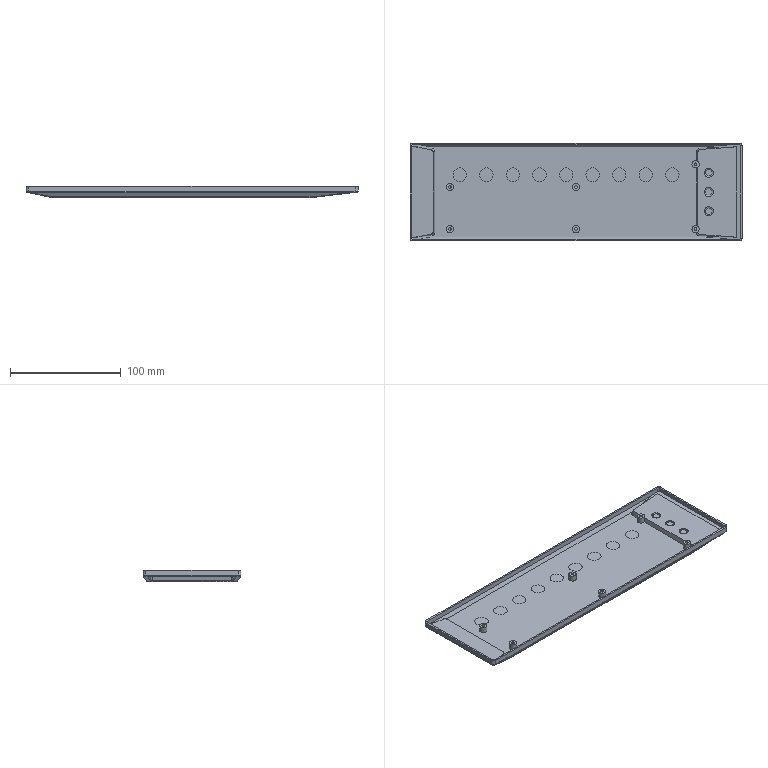NC program | NX | posted with a generic post | part box 300 x 88.5 x 10 mm
Whole program:
N10 G17 G21 G94 G90
(FIXED_CONTOUR_COPY_COPY , TOOL : D3R0.5)
N12 T09 M6
N14 G54
N16 G17 G0 G90 X-99.283 Y37.112 S9500 M3
N18 G43 Z30. H9
N20 Z3.6
N22 G94 G1 Z0.07 F1000.
N24 G3 X-99.023 Y36.962 R0.3
N26 G1 X-98.891 Z0.058 F2500.
N28 X117.392 Y36.963
N30 X117.548 Z0.07
N32 X117.664 Y36.874 Z0.069
N34 X117.542 Z0.057
N36 X117.392 Z0.045
N38 X117.321 Z0.044
N40 X-98.838 Y36.873
N42 X-99.15 Z0.071
N44 X-99.277 Y36.785
N46 X-98.953 Z0.041
N48 X-98.793 Z0.029
N50 X117.233 Y36.786
N52 X117.392 Z0.033
N54 X117.494 Z0.04
N56 X117.779 Z0.069
N58 X117.894 Y36.698 Z0.07
N60 X117.392 Z0.02
N62 X117.144 Z0.015
N64 X-98.749 Y36.697
N66 X-99.046 Z0.037
N68 X-99.404 Z0.072
N70 X-99.53 Y36.61
N72 X-99.041 Z0.025
N74 X-98.705 Z0.
N76 X117.056 Y36.611
N78 X117.409 Z0.009
N80 X118.009 Z0.07
N82 X118.123 Y36.524
N84 X117.35 Z-0.009
N86 X117.08 Z-0.014
N88 X-98.7 Y36.523
N90 X-98.777 Z-0.006
N92 X-99.046 Z0.014
N94 X-99.655 Z0.072
N96 X-99.78 Y36.436
N98 X-99.046 Z0.002
N100 X-98.865 Z-0.012
N102 X-98.7 Z-0.029
N104 X117.12 Y36.437
N106 X117.302 Z-0.025
N108 X118.236 Z0.071
N110 X118.349 Y36.351
N112 X117.255 Z-0.041
N114 X117.159 Z-0.043
N116 X-98.697 Y36.35
N118 X-98.951 Z-0.017
N120 X-99.046 Z-0.01
N122 X-99.904 Z0.072
N124 X-100.027 Y36.264
N126 X-98.67 Z-0.057
N128 X117.208 Y36.265
N130 X118.461 Z0.071
N132 X118.573 Y36.18 Z0.072
N134 X117.177 Z-0.072
N136 X-98.643 Y36.179
N138 X-100.15 Z0.072
N140 X-100.273 Y36.094 Z0.073
N142 X-98.616 Z-0.086
N144 X117.147 Y36.095
N146 X118.684 Z0.072
N148 X118.795 Y36.01
N150 X117.118 Z-0.1
N152 X-98.59 Y36.009
N154 X-100.395 Z0.073
N156 X-100.516 Y35.925
N158 X-98.563 Z-0.114
N160 X117.089 Y35.926
N162 X118.903 Z0.072
N164 X119.012 Y35.842
N166 X117.06 Z-0.128
N168 X-98.536 Y35.841
N170 X-100.636 Z0.073
N172 X-100.756 Y35.757
N174 X-98.51 Z-0.142
N176 X117.031
N178 X119.12 Z0.072
N180 X119.228 Y35.673
N182 X117.002 Z-0.156
N184 X-98.483 Y35.672
N186 X-100.876 Z0.073
N188 X-100.996 Y35.588
N190 X-98.456 Z-0.17
N192 X116.973 Y35.589
N194 X119.337 Z0.072
N196 X119.446 Y35.504 Z0.073
N198 X116.944 Z-0.184
N200 X-98.43
N202 X-101.116 Z0.073
N204 X-101.236 Y35.419
N206 X-98.403 Z-0.198
N208 X116.915 Y35.42
N210 X119.554 Z0.073
N212 X119.663 Y35.336
N214 X116.886 Z-0.212
N216 X-98.376 Y35.335
N218 X-101.356 Z0.073
N220 X-101.477 Y35.25
N222 X-98.35 Z-0.226
N224 X116.857 Y35.251
N226 X119.771 Z0.073
N228 X119.88 Y35.166
N230 X116.828 Z-0.24
N232 X-98.323 Z-0.241
N234 X-101.597 Z0.073
N236 X-101.717 Y35.081
N238 X-98.296 Z-0.255
N240 X116.799 Y35.082 Z-0.254
N242 X119.988 Z0.073
N244 X120.096 Y34.997
N246 X116.769 Z-0.269
N248 X-98.269 Y34.996
N250 X-101.838 Z0.073
N252 X-101.959 Y34.911
N254 X-98.243 Z-0.283
N256 X116.74 Y34.912
N258 X120.205 Z0.073
N260 X120.314 Y34.827
N262 X116.711 Z-0.297
N264 X-98.216
N266 X-102.079 Z0.073
N268 X-102.2 Y34.742
N270 X-98.189 Z-0.311
N272 X116.682 Y34.743
N274 X120.422 Z0.073
N276 X120.531 Y34.658
N278 X116.653 Z-0.325
N280 X-98.162 Y34.657
N282 X-102.321 Z0.073
N284 X-102.441 Y34.571
N286 X-98.135 Z-0.34
N288 X116.623 Y34.572 Z-0.339
N290 X120.64 Z0.073
N292 X120.749 Y34.486
N294 X116.594 Z-0.354
N296 X-98.107 Y34.485
N298 X-102.562 Z0.073
N300 X-102.684 Y34.399 Z0.072
N302 X-98.081 Z-0.368
N304 X116.564 Y34.4
N306 X120.858 Z0.072
N308 X120.969 Y34.313
N310 X116.534 Z-0.383
N312 X-98.053 Y34.312
N314 X-102.807 Z0.072
N316 X-102.93 Y34.224
N318 X-98.026 Z-0.397
N320 X116.504 Y34.225
N322 X121.079 Z0.072
N324 X121.191 Y34.138
N326 X116.474 Y34.137 Z-0.412
N328 X-97.998
N330 X-103.054 Z0.072
N332 X-103.178 Y34.048
N334 X-97.97 Z-0.427
N336 X116.443 Y34.049
N338 X121.302 Z0.072
N340 X121.414 Y33.961
N342 X116.413 Z-0.441
N344 X-97.942 Y33.96
N346 X-103.303 Z0.072
N348 X-103.427 Y33.871
N350 X-97.913 Z-0.456
N352 X116.382 Y33.872
N354 X121.527 Z0.072
N356 X121.638 Y33.784
N358 X116.352 Z-0.471
N360 X-97.886 Y33.783
N362 X-103.552 Z0.072
N364 X-103.676 Y33.695 Z0.071
N366 X-97.858 Z-0.486
N368 X116.321 Y33.696 Z-0.485
N370 X121.75 Z0.071
N372 X121.862 Y33.608
N374 X116.291 Z-0.5
N376 X-97.831 Y33.607
N378 X-103.799 Z0.071
N380 X-103.922 Y33.519
N382 X-97.803 Z-0.515
N384 X116.261 Y33.52
N386 X121.972 Z0.071
N388 X122.082 Y33.432
N390 X116.231 Z-0.529
N392 X-97.77 Y33.431
N394 X-104.044 Z0.071
N396 X-104.166 Y33.344 Z0.07
N398 X-97.894 Z-0.53
N400 X-97.735 Z-0.544
N402 X116.201 Y33.345
N404 X122.192 Z0.071
N406 X122.301 Y33.258 Z0.07
N408 X116.171 Z-0.558
N410 X-97.701 Y33.257
N412 X-97.947 Z-0.537
N414 X-104.288 Z0.07
N416 X-104.409 Y33.17
N418 X-97.999 Z-0.543
N420 X-97.666 Z-0.572
N422 X116.142 Y33.171
N424 X122.41 Z0.07
N426 X122.518 Y33.085
N428 X116.109 Z-0.586
N430 X-97.661 Y33.084 Z-0.587
N432 X-104.529 Z0.07
N434 X-104.65 Y32.998 Z0.069
N436 X-97.732 Z-0.592
N438 G3 X-97.472 Y33.148 R0.3
N440 G1 Z2.558
N442 G0 Z3.158
N444 X-98.024 Y32.941
N446 Z2.558
N448 G1 Z-0.592 F1000.
N450 G3 X-97.784 Y32.961 R0.24
N452 G1 X-97.773 Y32.97 F2500.
N454 X-97.855 Y32.912
N456 X-104.769 Z0.069
N458 X-104.888 Y32.827
N460 X-97.977 Z-0.592
N462 X-98.098 Y32.742
N464 X-105.007 Z0.069
N466 X-105.124 Y32.656 Z0.068
N468 X-98.221 Z-0.592
N470 X-98.345 Y32.57
N472 X-105.241 Z0.068
N474 X-105.284 Y32.537
N476 X-105.335 Y32.495 Z0.066
N478 X-105.353 Y32.479 Z0.067
N480 X-98.474 Z-0.592
N482 X-98.614 Y32.382
N484 X-105.177 Y32.381 Z0.037
N486 X-105.366 Z0.068
N488 X-105.369 Y32.282
N490 X-104.984 Z0.004
N492 X-98.755 Z-0.592
N494 X-98.897 Y32.183
N496 X-104.793 Z-0.027
N498 X-105.371 Z0.068
N500 X-105.372 Y32.084
N502 X-104.603 Z-0.059
N504 X-99.038 Z-0.592
N506 X-99.179 Y31.985
N508 X-104.413 Z-0.09
N510 X-105.373 Z0.068
N512 X-105.374 Y31.886 Z0.069
N514 X-104.222 Z-0.121
N516 X-102.751 Z-0.264
N518 X-99.319 Z-0.592
N520 X-99.46 Y31.787
N522 X-103.914 Z-0.166
N524 X-104.031 Z-0.153
N526 X-104.933 Z-0.004
N528 X-105.375 Z0.069
N530 X-105.376 Y31.688
N532 X-103.86 Z-0.181
N534 X-103.764 Z-0.193
N536 X-99.601 Z-0.592
N538 X-99.742 Y31.589
N540 X-103.442 Z-0.237
N542 X-103.651 Z-0.216
N544 X-105.377 Z0.069
N546 X-105.378 Y31.49
N548 X-103.46 Z-0.248
N550 X-103.256 Z-0.269
N552 X-99.883 Z-0.592
N554 X-100.024 Y31.391
N556 X-103.141 Z-0.294
N558 X-103.269 Z-0.28
N560 X-104.195 Z-0.127
N562 X-105.379 Z0.07
N564 X-105.38 Y31.292
N566 X-103.077 Z-0.312
N568 X-100.165 Z-0.592
N570 X-100.305 Y31.193
N572 X-102.887 Z-0.344
N574 X-105.381 Z0.07
N576 X-105.382 Y31.093
N578 X-102.698 Z-0.377
N580 X-100.445 Z-0.592
N582 X-100.585 Y30.994
N584 X-102.505 Z-0.409
N586 X-105.383 Z0.07
N588 X-105.384 Y30.895
N590 X-102.315 Z-0.441
N592 X-100.725 Z-0.592
N594 X-100.865 Y30.796
N596 X-102.124 Z-0.472
N598 X-105.385 Z0.071
N600 X-105.386 Y30.697
N602 X-101.934 Z-0.504
N604 X-101.006 Z-0.592
N606 X-101.145 Y30.598
N608 X-101.744 Z-0.535
N610 X-105.387 Z0.071
N612 Y30.499
N614 X-101.554 Z-0.567
N616 X-101.285 Z-0.593
N618 X-101.402 Y30.416 Z-0.592
N620 Y30.4
N622 X-105.388 Y30.399 Z0.071
N624 X-105.389 Y30.299
N626 X-101.402 Y30.3 Z-0.592
N628 X-101.403 Y30.2
N630 X-105.389 Y30.199 Z0.072
N632 X-105.39 Y30.099
N634 X-101.403 Y30.1 Z-0.592
N636 Y30.
N638 X-105.391 Y29.999 Z0.072
N640 Y29.899
N642 X-101.404 Y29.9 Z-0.592
N644 Y29.8
N646 X-105.392 Y29.799 Z0.072
N648 X-105.393 Y29.7
N650 X-101.405 Z-0.592
N652 Y29.6
N654 X-105.393 Z0.072
N656 X-105.394 Y29.5
N658 X-101.405 Z-0.592
N660 Y29.4
N662 X-105.395 Z0.072
N664 Y29.3 Z0.073
N666 X-101.405 Z-0.592
N668 X-101.406 Y29.2
N670 X-105.396 Z0.073
N672 X-105.397 Y29.1
N674 X-101.406 Z-0.592
N676 Y29.
N678 X-105.397 Z0.073
N680 X-105.398 Y28.9
N682 X-101.406 Z-0.592
N684 X-101.407 Y28.8
N686 X-105.399 Z0.073
N688 Y28.7
N690 X-101.407 Z-0.592
N692 Y28.6
N694 X-105.4 Z0.073
N696 Y28.5
N698 X-101.407 Z-0.592
N700 Y28.4
N702 X-105.4 Z0.073
N704 X-105.401 Y28.3
N706 X-101.408 Z-0.592
N708 Y28.2
N710 X-105.401 Z0.074
N712 X-105.402 Y28.1
N714 X-101.408 Z-0.592
N716 Y28. Z-0.591
N718 X-105.402 Z0.074
N720 Y27.9
N722 X-101.409 Z-0.591
N724 Y27.8
N726 X-105.403 Z0.074
N728 Y27.7
N730 X-101.409 Z-0.591
N732 Y27.6
N734 X-105.403 Z0.074
N736 X-105.404 Y27.5
N738 X-101.409 Z-0.591
N740 Y27.4
N742 X-105.404 Z0.074
N744 X-105.405 Y27.3
N746 X-101.409 Z-0.591
N748 Y27.2
N750 X-105.405 Z0.074
N752 Y27.1
N754 X-101.409 Z-0.591
N756 Y27.
N758 X-105.406 Z0.074
N760 Y26.9
N762 X-101.409 Z-0.591
N764 Y26.8
N766 X-105.406 Z0.074
N768 Y26.7
N770 X-101.409 Z-0.591
N772 X-101.41 Y26.6
N774 X-105.406 Z0.074
N776 X-105.407 Y26.5
N778 X-101.41 Z-0.591
N780 Y26.4
N782 X-105.407 Z0.074
N784 Y26.3
N786 X-101.41 Z-0.591
N788 Y26.2
N790 X-105.407 Z0.075
N792 Y26.1
N794 X-101.41 Z-0.591
N796 Y26.
N798 X-105.407 Z0.075
N800 X-105.408 Y25.9
N802 X-101.41 Z-0.591
N804 Y25.8
N806 X-105.408 Z0.075
N808 Y25.7
N810 X-101.41 Z-0.591
N812 Y25.6
N814 X-105.408 Z0.075
N816 Y25.5
N818 X-101.41 Z-0.591
N820 Y25.4
N822 X-105.408 Z0.075
N824 X-105.409 Y25.3
N826 X-101.41 Z-0.591
N828 Y25.2
N830 X-105.409 Z0.075
N832 Y25.1
N834 X-101.41 Z-0.591
N836 Y25.
N838 X-105.409 Z0.075
N840 Y24.9
N842 X-101.41 Z-0.591
N844 Y24.8
N846 X-105.409 Z0.075
N848 X-105.41 Y24.7
N850 X-101.411 Z-0.591
N852 Y24.6
N854 X-105.41 Z0.075
N856 Y24.5
N858 X-101.411 Z-0.591
N860 Y24.4
N862 X-105.41 Z0.075
N864 Y24.3
N866 X-101.411 Z-0.591
N868 Y24.2
N870 X-105.41 Z0.075
N872 Y24.1
N874 X-101.411 Z-0.591
N876 Y24.
N878 X-105.41 Z0.075
N880 Y23.9
N882 X-101.411 Z-0.591
N884 Y23.8
N886 X-105.41 Z0.075
N888 Y23.7
N890 X-101.411 Z-0.591
N892 Y23.6
N894 X-105.41 Z0.075
N896 Y23.5
N898 X-101.411 Z-0.591
N900 Y23.4
N902 X-105.41 Z0.075
N904 Y23.3
N906 X-101.411 Z-0.591
N908 Y23.2
N910 X-105.41 Z0.075
N912 Y23.1
N914 X-101.411 Z-0.591
N916 Y23.
N918 X-105.41 Z0.075
N920 Y22.9
N922 X-101.411 Z-0.591
N924 X-101.412 Y22.8
N926 X-105.41 Z0.075
N928 Y22.7
N930 X-101.412 Z-0.591
N932 Y22.6
N934 X-105.41 Z0.075
N936 Y22.5
N938 X-101.412 Z-0.591
N940 Y22.4
N942 X-105.41 Z0.075
N944 Y22.3
N946 X-101.412 Z-0.591
N948 Y22.2
N950 X-105.41 Z0.075
N952 Y22.1
N954 X-101.412 Z-0.591
N956 Y22.
N958 X-105.41 Z0.075
N960 Y21.9
N962 X-101.412 Z-0.591
N964 Y21.8
N966 X-105.41 Z0.075
N968 Y21.7
N970 X-101.412 Z-0.591
N972 Y21.6
N974 X-105.41 Z0.075
N976 Y21.5
N978 X-101.412 Z-0.591
N980 Y21.4
N982 X-105.41 Z0.075
N984 Y21.3
N986 X-101.412 Z-0.591
N988 Y21.2
N990 X-105.41 Z0.075
N992 Y21.1
N994 X-101.412 Z-0.591
N996 Y21.
N998 X-105.41 Z0.075
N1000 Y20.9
N1002 X-101.412 Z-0.591
N1004 Y20.8
N1006 X-105.41 Z0.075
N1008 Y20.7
N1010 X-101.412 Z-0.591
N1012 Y20.6
N1014 X-105.41 Z0.075
N1016 Y20.5
N1018 X-101.412 Z-0.591
N1020 X-101.411 Y20.4
N1022 X-105.41 Z0.075
N1024 Y20.3
N1026 X-101.411 Z-0.591
N1028 Y20.2
N1030 X-105.41 Z0.075
N1032 Y20.1
N1034 X-101.411 Z-0.591
N1036 Y20.
N1038 X-105.41 Z0.075
N1040 Y19.9
N1042 X-101.411 Z-0.591
N1044 Y19.8
N1046 X-105.41 Z0.075
N1048 Y19.7
N1050 X-101.411 Z-0.591
N1052 Y19.6
N1054 X-105.41 Z0.075
N1056 Y19.5
N1058 X-101.411 Z-0.591
N1060 Y19.4
N1062 X-105.41 Z0.075
N1064 Y19.3
N1066 X-101.411 Z-0.591
N1068 Y19.2
N1070 X-105.41 Z0.075
N1072 Y19.1
N1074 X-101.411 Z-0.591
N1076 Y19.
N1078 X-105.41 Z0.075
N1080 Y18.9
N1082 X-101.411 Z-0.591
N1084 Y18.8
N1086 X-105.41 Z0.075
N1088 Y18.7
N1090 X-101.411 Z-0.591
N1092 Y18.6
N1094 X-105.41 Z0.075
N1096 Y18.5
N1098 X-101.411 Z-0.591
N1100 Y18.4
N1102 X-105.41 Z0.075
N1104 Y18.3
N1106 X-101.411 Z-0.591
N1108 Y18.2
N1110 X-105.411 Z0.075
N1112 Y18.1
N1114 X-101.411 Z-0.591
N1116 Y18.
N1118 X-105.411 Z0.075
N1120 Y17.9
N1122 X-101.411 Z-0.591
N1124 Y17.8
N1126 X-105.411 Z0.075
N1128 Y17.7
N1130 X-101.411 Z-0.591
N1132 Y17.6
N1134 X-105.411 Z0.075
N1136 Y17.5
N1138 X-101.411 Z-0.591
N1140 Y17.4
N1142 X-105.411 Z0.075
N1144 Y17.3
N1146 X-101.411 Z-0.591
N1148 Y17.2
N1150 X-105.411 Z0.075
N1152 Y17.1
N1154 X-101.411 Z-0.591
N1156 Y17.
N1158 X-105.411 Z0.075
N1160 Y16.9
N1162 X-101.411 Z-0.591
N1164 Y16.8
N1166 X-105.411 Z0.075
N1168 Y16.7
N1170 X-101.411 Z-0.591
N1172 Y16.6
N1174 X-105.411 Z0.075
N1176 Y16.5
N1178 X-101.411 Z-0.591
N1180 Y16.4
N1182 X-105.411 Z0.075
N1184 Y16.3
N1186 X-101.411 Z-0.591
N1188 Y16.2
N1190 X-105.411 Z0.075
N1192 Y16.1
N1194 X-101.411 Z-0.591
N1196 Y16.
N1198 X-105.411 Z0.075
N1200 Y15.9
N1202 X-101.411 Z-0.591
N1204 Y15.8
N1206 X-105.411 Z0.075
N1208 Y15.7
N1210 X-101.411 Z-0.591
N1212 Y15.6
N1214 X-105.411 Z0.075
N1216 Y15.5
N1218 X-101.411 Z-0.591
N1220 Y15.4
N1222 X-105.411 Z0.075
N1224 Y15.3
N1226 X-101.411 Z-0.591
N1228 Y15.2
N1230 X-105.411 Z0.075
N1232 Y15.1
N1234 X-101.411 Z-0.591
N1236 Y15.
N1238 X-105.411 Z0.075
N1240 Y14.9
N1242 X-101.411 Z-0.591
N1244 Y14.8
N1246 X-105.411 Z0.075
N1248 Y14.7
N1250 X-101.411 Z-0.591
N1252 Y14.6
N1254 X-105.411 Z0.075
N1256 Y14.5
N1258 X-101.411 Z-0.591
N1260 Y14.4
N1262 X-105.411 Z0.075
N1264 Y14.3
N1266 X-101.411 Z-0.591
N1268 Y14.2
N1270 X-105.411 Z0.075
N1272 Y14.1
N1274 X-101.411 Z-0.591
N1276 Y14.
N1278 X-105.411 Z0.075
N1280 Y13.9
N1282 X-101.411 Z-0.591
N1284 Y13.8
N1286 X-105.411 Z0.075
N1288 Y13.7
N1290 X-101.411 Z-0.591
N1292 Y13.6
N1294 X-105.411 Z0.075
N1296 X-105.41 Y13.5
N1298 X-101.411 Z-0.591
N1300 Y13.4
N1302 X-105.41 Z0.075
N1304 Y13.3
N1306 X-101.411 Z-0.591
N1308 Y13.2
N1310 X-105.41 Z0.075
N1312 Y13.1
N1314 X-101.411 Z-0.591
N1316 Y13.
N1318 X-105.41 Z0.075
N1320 Y12.9
N1322 X-101.411 Z-0.591
N1324 Y12.8
N1326 X-105.41 Z0.075
N1328 Y12.7
N1330 X-101.411 Z-0.591
N1332 Y12.6
N1334 X-105.41 Z0.075
N1336 Y12.501
N1338 X-101.411 Y12.5 Z-0.591
N1340 Y12.4
N1342 X-105.41 Z0.075
N1344 Y12.3
N1346 X-101.411 Z-0.591
N1348 Y12.2
N1350 X-105.41 Z0.075
N1352 Y12.1
N1354 X-101.411 Z-0.591
N1356 Y12.
N1358 X-105.41 Z0.075
N1360 Y11.9
N1362 X-101.411 Z-0.591
N1364 Y11.8
N1366 X-105.41 Z0.075
N1368 Y11.7
N1370 X-101.411 Z-0.591
N1372 Y11.6
N1374 X-105.41 Z0.075
N1376 Y11.5
N1378 X-101.411 Z-0.591
N1380 Y11.4
N1382 X-105.41 Z0.075
N1384 Y11.3
N1386 X-101.411 Z-0.591
N1388 Y11.2
N1390 X-105.41 Z0.075
N1392 X-105.409 Y11.1
N1394 X-101.411 Z-0.591
N1396 Y11.
N1398 X-105.409 Z0.075
N1400 Y10.9
N1402 X-101.411 Z-0.591
N1404 Y10.8
N1406 X-105.409 Z0.075
N1408 Y10.7
N1410 X-101.411 Z-0.591
N1412 Y10.6
N1414 X-105.409 Z0.075
N1416 Y10.5
N1418 X-101.411 Z-0.591
N1420 Y10.4
N1422 X-105.409 Z0.075
N1424 Y10.3
N1426 X-101.411 Z-0.591
N1428 Y10.2
N1430 X-105.409 Z0.075
N1432 Y10.1
N1434 X-101.411 Z-0.591
N1436 Y10.
N1438 X-105.409 Z0.075
N1440 Y9.9
N1442 X-101.411 Z-0.591
N1444 Y9.8
N1446 X-105.409 Z0.075
N1448 Y9.7
N1450 X-101.411 Z-0.591
N1452 Y9.6
N1454 X-105.409 Z0.075
N1456 Y9.5
N1458 X-101.411 Z-0.591
N1460 Y9.4
N1462 X-105.409 Z0.075
N1464 Y9.3
N1466 X-101.41 Z-0.591
N1468 Y9.2
N1470 X-105.409 Z0.075
N1472 Y9.1
N1474 X-101.41 Z-0.591
N1476 Y9.
N1478 X-105.409 Z0.075
N1480 X-105.408 Y8.9
N1482 X-101.41 Z-0.591
N1484 Y8.8
N1486 X-105.408 Z0.075
N1488 Y8.7
N1490 X-101.41 Z-0.591
N1492 X-101.409 Y8.6
N1494 X-105.407 Z0.075
N1496 Y8.5
N1498 X-101.409 Z-0.591
N1500 Y8.4
N1502 X-105.407 Z0.074
N1504 Y8.3
N1506 X-101.409 Z-0.591
N1508 Y8.2
N1510 X-105.406 Z0.074
N1512 Y8.1
N1514 X-101.409 Z-0.592
N1516 X-101.408 Y8.
N1518 X-105.406 Z0.074
N1520 Y7.9
N1522 X-101.408 Z-0.592
N1524 Y7.8
N1526 X-105.405 Z0.074
N1528 Y7.7
N1530 X-101.408 Z-0.592
N1532 Y7.6
N1534 X-105.405 Z0.074
N1536 Y7.5
N1538 X-101.408 Z-0.592
N1540 X-101.407 Y7.4
N1542 X-105.404 Z0.074
N1544 Y7.3
N1546 X-101.407 Z-0.592
N1548 Y7.2
N1550 X-105.404 Z0.074
N1552 Y7.1
N1554 X-101.407 Z-0.592
N1556 Y7.
N1558 X-105.403 Z0.074
N1560 Y6.9
N1562 X-101.407 Z-0.592
N1564 Y6.8
N1566 X-105.403 Z0.074
N1568 Y6.7
N1570 X-101.406 Z-0.592
N1572 Y6.6
N1574 X-105.402 Z0.074
N1576 Y6.5
N1578 X-101.406 Z-0.592
N1580 Y6.4
N1582 X-105.401 Z0.074
N1584 Y6.3 Z0.073
N1586 X-101.406 Z-0.592
N1588 Y6.2
N1590 X-105.4 Z0.073
N1592 X-105.399 Y6.1
N1594 X-101.405 Z-0.592
N1596 Y6.
N1598 X-105.399 Z0.073
N1600 X-105.398 Y5.9
N1602 X-101.405 Z-0.592
N1604 Y5.8
N1606 X-105.398 Z0.073
N1608 X-105.397 Y5.7
N1610 X-101.404 Z-0.592
N1612 Y5.6
N1614 X-105.397 Z0.073
N1616 X-105.396 Y5.5
N1618 X-101.403 Z-0.592
N1620 Y5.4
N1622 X-105.395 Z0.073
N1624 Y5.3 Z0.072
N1626 X-101.402 Z-0.592
N1628 Y5.2
N1630 X-105.394 Z0.072
N1632 Y5.1
N1634 X-101.401 Z-0.592
N1636 Y5.
N1638 X-105.393 Z0.072
N1640 Y4.9
N1642 X-101.4 Z-0.592
N1644 Y4.8
N1646 X-105.392 Z0.072
N1648 X-105.391 Y4.7
N1650 X-101.4 Z-0.592
N1652 X-101.399 Y4.6
N1654 X-105.39 Z0.072
N1656 X-105.389 Y4.5 Z0.071
N1658 X-101.399 Z-0.592
N1660 X-101.398 Y4.4 Z-0.593
N1662 X-105.388 Z0.071
N1664 X-105.387 Y4.3
N1666 X-101.397 Z-0.593
N1668 Y4.223 Z-0.594
N1670 X-101.369 Y4.2 Z-0.595
N1672 X-101.426 Z-0.589
N1674 X-105.386 Z0.071
N1676 X-105.385 Y4.108
N1678 X-101.61 Z-0.557
N1680 X-101.254 Z-0.594
N1682 X-101.138 Y4.016
N1684 X-101.798 Z-0.526
N1686 X-105.384 Z0.071
N1688 Y3.925 Z0.07
N1690 X-101.988 Z-0.495
N1692 X-101.022 Z-0.593
N1694 X-100.906 Y3.833
N1696 X-102.176 Z-0.464
N1698 X-105.383 Z0.07
N1700 X-105.382 Y3.742
N1702 X-102.363 Z-0.433
N1704 X-100.79 Z-0.593
N1706 X-100.674 Y3.65
N1708 X-102.548 Z-0.402
N1710 X-105.381 Z0.07
N1712 X-105.38 Y3.558
N1714 X-102.724 Z-0.371
N1716 X-100.557 Z-0.593
N1718 X-100.44 Y3.465
N1720 X-102.907 Z-0.34
N1722 X-105.379 Z0.07
N1724 X-105.378 Y3.372 Z0.069
N1726 X-103.325 Z-0.271
N1728 X-103.098 Z-0.308
N1730 X-100.322 Z-0.593
N1732 X-100.204 Y3.279
N1734 X-103.29 Z-0.276
N1736 X-103.894 Z-0.177
N1738 X-105.377 Z0.069
N1740 Y3.185
N1742 X-103.548 Z-0.234
N1744 X-103.484 Z-0.244
N1746 X-100.085 Z-0.593
N1748 X-99.966 Y3.091
N1750 X-103.678 Z-0.211
N1752 X-105.376 Z0.069
N1754 X-105.375 Y2.998
N1756 X-103.873 Z-0.179
N1758 X-99.846 Z-0.593
N1760 X-99.726 Y2.904
N1762 X-104.068 Z-0.146
N1764 X-105.374 Z0.069
N1766 X-105.373 Y2.81 Z0.068
N1768 X-104.263 Z-0.114
N1770 X-99.607 Z-0.593
N1772 X-99.487 Y2.717
N1774 X-104.458 Z-0.082
N1776 X-105.372 Z0.068
N1778 X-105.371 Y2.624
N1780 X-104.652 Z-0.05
N1782 X-99.368 Z-0.593
N1784 X-99.249 Y2.53
N1786 X-104.847 Z-0.018
N1788 X-105.371 Z0.068
N1790 X-105.369 Y2.437 Z0.067
N1792 X-105.039 Z0.013
N1794 X-99.13 Z-0.593
N1796 X-99.01 Y2.344
N1798 X-105.229 Z0.045
N1800 X-105.367 Z0.066
N1802 X-105.365 Y2.278 Z0.065
N1804 X-105.347 Y2.263 Z0.062
N1806 X-105.331 Y2.251 Z0.063
N1808 X-105.279 Z0.062
N1810 X-98.891 Z-0.593
N1812 X-98.773 Y2.158
N1814 X-105.219 Z0.068
N1816 X-105.104 Y2.064
N1818 X-98.653 Z-0.593
N1820 X-98.533 Y1.971
N1822 X-104.986 Z0.069
N1824 X-104.869 Y1.877
N1826 X-98.413 Z-0.593
N1828 X-98.293 Y1.784
N1830 X-104.752 Z0.069
N1832 X-104.635 Y1.691
N1834 X-98.173 Z-0.593
N1836 X-98.053 Y1.598
N1838 X-104.518 Z0.07
N1840 X-104.401 Y1.505
N1842 X-97.934 Z-0.593
N1844 X-97.815 Y1.413
N1846 X-104.285 Z0.07
N1848 X-104.169 Y1.321
N1850 X-97.696 Z-0.593
N1852 X-97.611 Y1.254 Z-0.591
N1854 X-97.575 Z-0.593
N1856 X-93.852 Y1.243 Z-0.592
N1858 X-89.696 Y1.239 Z-0.591
N1860 X10.036 Y1.238
N1862 X-97.585 Z-0.59
N1864 X-97.656 Z-0.586
N1866 X-104.065 Z0.071
N1868 G3 X-104.324 Y1.088 R0.3
N1870 G1 Z3.6
N1872 G0 Z30.
N1874 X-98.024 Y32.941
N1876 Z3.
N1878 G1 Z-0.592 F1000.
N1880 G3 X-97.784 Y32.961 R0.24
N1882 G1 X-97.659 Y33.049 F2500.
N1884 X-94.543 Y33.058
N1886 X-90.389 Y33.061 Z-0.591
N1888 X109.773 Y33.06
N1890 X113.235 Y33.055 Z-0.592
N1892 X116.1 Y33.046 Z-0.593
N1894 X116.162 Y32.999
N1896 X122.626 Z0.07
N1898 X122.734 Y32.913 Z0.069
N1900 X116.272 Z-0.593
N1902 X116.382 Y32.828
N1904 X122.841 Z0.069
N1906 X122.948 Y32.743
N1908 X116.491 Z-0.593
N1910 X116.601 Y32.657
N1912 X123.055 Z0.069
N1914 X123.164 Y32.571 Z0.068
N1916 X116.713 Z-0.593
N1918 X116.829 Y32.48
N1920 X123.274 Z0.068
N1922 X123.364 Y32.405 Z0.064
N1924 X123.365 Y32.382
N1926 X123.311 Z0.058
N1928 X123.28 Z0.056
N1930 X116.955 Z-0.593
N1932 X117.082 Y32.283
N1934 X123.115 Z0.026
N1936 X123.31 Z0.059
N1938 X123.368 Z0.066
N1940 X123.37 Y32.184 Z0.067
N1942 X122.912 Z-0.008
N1944 X117.21 Z-0.593
N1946 X117.336 Y32.085
N1948 X122.706 Z-0.042
N1950 X123.371 Z0.068
N1952 X123.372 Y31.986
N1954 X122.5 Z-0.075
N1956 X117.462 Z-0.593
N1958 X117.589 Y31.887
N1960 X122.293 Z-0.109
N1962 X123.373 Z0.068
N1964 X123.374 Y31.788 Z0.069
N1966 X122.24 Z-0.12
N1968 X122.087 Z-0.143
N1970 X117.715 Z-0.593
N1972 X117.841 Y31.689
N1974 X121.881 Z-0.177
N1976 X122.148 Z-0.135
N1978 X123.375 Z0.069
N1980 X123.376 Y31.59
N1982 X121.753 Z-0.2
N1984 X121.632 Z-0.216
N1986 X117.968 Z-0.593
N1988 X118.094 Y31.491
N1990 X121.469 Z-0.246
N1992 X121.949 Z-0.168
N1994 X123.377 Z0.069
N1996 X123.378 Y31.392
N1998 X121.503 Z-0.243
N2000 X121.264 Z-0.28
N2002 X118.221 Z-0.593
N2004 X118.347 Y31.292
N2006 X121.06 Z-0.315
N2008 X121.403 Z-0.259
N2010 X123.379 Z0.07
N2012 X123.38 Y31.193
N2014 X120.857 Z-0.349
N2016 X118.473 Z-0.593
N2018 X118.599 Y31.094
N2020 X120.665 Z-0.381
N2022 X123.381 Z0.07
N2024 X123.382 Y30.995
N2026 X120.475 Z-0.414
N2028 X118.724 Z-0.593
N2030 X118.849 Y30.896
N2032 X120.272 Z-0.448
N2034 X123.383 Z0.07
N2036 X123.384 Y30.797 Z0.071
N2038 X120.068 Z-0.482
N2040 X118.975 Z-0.593
N2042 X119.1 Y30.698
N2044 X119.864 Z-0.516
N2046 X123.385 Z0.071
N2048 X123.386 Y30.599
N2050 X119.66 Z-0.549
N2052 X119.226 Z-0.593
N2054 X119.354 Y30.5
N2056 X119.47 Z-0.58
N2058 X123.387 Z0.071
N2060 X123.388 Y30.4
N2062 X119.398 Z-0.592
N2064 X119.399 Y30.3
N2066 X123.389 Z0.071
N2068 Y30.2 Z0.072
N2070 X119.399 Z-0.592
N2072 X119.4 Y30.1
N2074 X123.39 Z0.072
N2076 X123.391 Y30.
N2078 X119.4 Z-0.592
N2080 X119.401 Y29.9
N2082 X123.391 Z0.072
N2084 X123.392 Y29.8
N2086 X119.401 Z-0.592
N2088 Y29.7
N2090 X123.393 Z0.072
N2092 Y29.6
N2094 X119.402 Z-0.592
N2096 Y29.5
N2098 X123.394 Z0.072
N2100 X123.395 Y29.4
N2102 X119.402 Z-0.592
N2104 X119.403 Y29.3
N2106 X123.395 Z0.073
N2108 X123.396 Y29.2
N2110 X119.403 Z-0.592
N2112 Y29.1
N2114 X123.397 Z0.073
N2116 Y29.
N2118 X119.404 Z-0.592
N2120 Y28.9
N2122 X123.398 Z0.073
N2124 Y28.8
N2126 X119.404 Z-0.592
N2128 X119.405 Y28.7
N2130 X123.399 Z0.073
N2132 X123.4 Y28.6
N2134 X119.405 Z-0.592
N2136 Y28.5
N2138 X123.4 Z0.073
N2140 X123.401 Y28.4 Z0.074
N2142 X119.406 Z-0.592
N2144 Y28.3
N2146 X123.401 Z0.074
N2148 X123.402 Y28.2
N2150 X119.406 Z-0.592
N2152 X119.407 Y28.1
N2154 X123.402 Z0.074
N2156 Y28.
N2158 X119.407 Z-0.592
N2160 Y27.9
N2162 X123.403 Z0.074
N2164 Y27.8
N2166 X119.407 Z-0.592
N2168 Y27.7
N2170 X123.403 Z0.074
N2172 X123.404 Y27.6
N2174 X119.407 Z-0.592
N2176 Y27.5
N2178 X123.404 Z0.074
N2180 Y27.4
N2182 X119.408 Z-0.592
N2184 Y27.3
N2186 X123.405 Z0.074
N2188 Y27.2
N2190 X119.408 Z-0.592
N2192 Y27.1
N2194 X123.405 Z0.074
N2196 X123.406 Y27.
N2198 X119.408 Z-0.592
N2200 Y26.9
N2202 X123.406 Z0.074
N2204 Y26.8
N2206 X119.408 Z-0.592
N2208 X119.409 Y26.7
N2210 X123.406 Z0.074
N2212 Y26.6
N2214 X119.409 Z-0.591
N2216 Y26.5
N2218 X123.407 Z0.074
N2220 Y26.4
N2222 X119.409 Z-0.591
N2224 Y26.3
N2226 X123.407 Z0.074
N2228 Y26.2 Z0.075
N2230 X119.409 Z-0.591
N2232 Y26.1
N2234 X123.407 Z0.075
N2236 Y26.
N2238 X119.409 Z-0.591
N2240 X119.41 Y25.9
N2242 X123.408 Z0.075
N2244 Y25.8
N2246 X119.41 Z-0.591
N2248 Y25.7
N2250 X123.408 Z0.075
N2252 Y25.6
N2254 X119.41 Z-0.591
N2256 Y25.5
N2258 X123.408 Z0.075
N2260 Y25.4
N2262 X119.41 Z-0.591
N2264 Y25.3
N2266 X123.408 Z0.075
N2268 X123.409 Y25.2
N2270 X119.41 Z-0.591
N2272 X119.411 Y25.1
N2274 X123.409 Z0.075
N2276 Y25.
N2278 X119.411 Z-0.591
N2280 Y24.9
N2282 X123.409 Z0.075
N2284 Y24.8
N2286 X119.411 Z-0.591
N2288 Y24.7
N2290 X123.409 Z0.075
N2292 X123.41 Y24.6
N2294 X119.411 Z-0.591
N2296 Y24.5
N2298 X123.41 Z0.075
N2300 Y24.4
N2302 X119.411 Z-0.591
N2304 Y24.3
N2306 X123.41 Z0.075
N2308 Y24.2
N2310 X119.411 Z-0.591
N2312 Y24.1
N2314 X123.41 Z0.075
N2316 Y24.
N2318 X119.411 Z-0.591
N2320 Y23.9
N2322 X123.41 Z0.075
N2324 Y23.8
N2326 X119.411 Z-0.591
N2328 Y23.7
N2330 X123.41 Z0.075
N2332 Y23.6
N2334 X119.411 Z-0.591
N2336 Y23.5
N2338 X123.41 Z0.075
N2340 Y23.4
N2342 X119.411 Z-0.591
N2344 Y23.3
N2346 X123.41 Z0.075
N2348 Y23.2
N2350 X119.411 Z-0.591
N2352 Y23.1
N2354 X123.41 Z0.075
N2356 Y23.
N2358 X119.411 Z-0.591
N2360 Y22.9
N2362 X123.41 Z0.075
N2364 Y22.8
N2366 X119.411 Z-0.591
N2368 Y22.7
N2370 X123.41 Z0.075
N2372 Y22.6
N2374 X119.411 Z-0.591
N2376 Y22.5
N2378 X123.41 Z0.075
N2380 Y22.4
N2382 X119.411 Z-0.591
N2384 Y22.3
N2386 X123.41 Z0.075
N2388 Y22.2
N2390 X119.411 Z-0.591
N2392 Y22.1
N2394 X123.41 Z0.075
N2396 Y22.
N2398 X119.411 Z-0.591
N2400 Y21.9
N2402 X123.41 Z0.075
N2404 Y21.8
N2406 X119.411 Z-0.591
N2408 Y21.7
N2410 X123.41 Z0.075
N2412 Y21.6
N2414 X119.411 Z-0.591
N2416 Y21.5
N2418 X123.41 Z0.075
N2420 Y21.4
N2422 X119.411 Z-0.591
N2424 Y21.3
N2426 X123.41 Z0.075
N2428 Y21.2
N2430 X119.411 Z-0.591
N2432 Y21.1
N2434 X123.41 Z0.075
N2436 Y21.
N2438 X119.411 Z-0.591
N2440 Y20.9
N2442 X123.41 Z0.075
N2444 Y20.8
N2446 X119.411 Z-0.591
N2448 Y20.7
N2450 X123.41 Z0.075
N2452 Y20.6
N2454 X119.411 Z-0.591
N2456 Y20.5
N2458 X123.41 Z0.075
N2460 Y20.4
N2462 X119.411 Z-0.591
N2464 Y20.3
N2466 X123.41 Z0.075
N2468 Y20.2
N2470 X119.411 Z-0.591
N2472 Y20.1
N2474 X123.41 Z0.075
N2476 Y20.
N2478 X119.411 Z-0.591
N2480 Y19.9
N2482 X123.41 Z0.075
N2484 Y19.8
N2486 X119.411 Z-0.591
N2488 Y19.7
N2490 X123.41 Z0.075
N2492 Y19.6
N2494 X119.411 Z-0.591
N2496 Y19.5
N2498 X123.41 Z0.075
N2500 Y19.4
N2502 X119.411 Z-0.591
N2504 Y19.3
N2506 X123.41 Z0.075
N2508 Y19.2
N2510 X119.411 Z-0.591
N2512 Y19.1
N2514 X123.41 Z0.075
N2516 Y19.
N2518 X119.411 Z-0.591
N2520 Y18.9
N2522 X123.41 Z0.075
N2524 Y18.8
N2526 X119.411 Z-0.591
N2528 Y18.7
N2530 X123.41 Z0.075
N2532 Y18.6
N2534 X119.411 Z-0.591
N2536 Y18.5
N2538 X123.41 Z0.075
N2540 Y18.4
N2542 X119.411 Z-0.591
N2544 Y18.3
N2546 X123.41 Z0.075
N2548 Y18.2
N2550 X119.411 Z-0.591
N2552 Y18.1
N2554 X123.41 Z0.075
N2556 Y18.
N2558 X119.411 Z-0.591
N2560 Y17.9
N2562 X123.41 Z0.075
N2564 Y17.8
N2566 X119.411 Z-0.591
N2568 Y17.7
N2570 X123.41 Z0.075
N2572 Y17.6
N2574 X119.411 Z-0.591
N2576 Y17.5
N2578 X123.41 Z0.075
N2580 Y17.4
N2582 X119.411 Z-0.591
N2584 Y17.3
N2586 X123.41 Z0.075
N2588 Y17.2
N2590 X119.411 Z-0.591
N2592 Y17.1
N2594 X123.41 Z0.075
N2596 Y17.
N2598 X119.411 Z-0.591
N2600 Y16.9
N2602 X123.41 Z0.075
N2604 Y16.8
N2606 X119.411 Z-0.591
N2608 Y16.7
N2610 X123.41 Z0.075
N2612 Y16.6
N2614 X119.411 Z-0.591
N2616 Y16.5
N2618 X123.41 Z0.075
N2620 Y16.4
N2622 X119.411 Z-0.591
N2624 Y16.3
N2626 X123.41 Z0.075
N2628 Y16.2
N2630 X119.411 Z-0.591
N2632 Y16.1
N2634 X123.41 Z0.075
N2636 Y16.
N2638 X119.411 Z-0.591
N2640 Y15.9
N2642 X123.41 Z0.075
N2644 Y15.8
N2646 X119.411 Z-0.591
N2648 Y15.7
N2650 X123.41 Z0.075
N2652 Y15.601
N2654 X119.411 Y15.6 Z-0.591
N2656 Y15.5
N2658 X123.41 Z0.075
N2660 Y15.4
N2662 X119.411 Z-0.591
N2664 Y15.3
N2666 X123.41 Z0.075
N2668 Y15.2
N2670 X119.411 Z-0.591
N2672 Y15.1
N2674 X123.41 Z0.075
N2676 Y15.
N2678 X119.411 Z-0.591
N2680 Y14.9
N2682 X123.41 Z0.075
N2684 Y14.8
N2686 X119.411 Z-0.591
N2688 Y14.7
N2690 X123.41 Z0.075
N2692 Y14.6
N2694 X119.411 Z-0.591
N2696 Y14.5
N2698 X123.41 Z0.075
N2700 Y14.4
N2702 X119.411 Z-0.591
N2704 Y14.3
N2706 X123.41 Z0.075
N2708 Y14.2
N2710 X119.411 Z-0.591
N2712 Y14.1
N2714 X123.41 Z0.075
N2716 Y14.
N2718 X119.411 Z-0.591
N2720 Y13.9
N2722 X123.41 Z0.075
N2724 Y13.8
N2726 X119.411 Z-0.591
N2728 Y13.7
N2730 X123.41 Z0.075
N2732 Y13.6
N2734 X119.411 Z-0.591
N2736 Y13.5
N2738 X123.41 Z0.075
N2740 Y13.4
N2742 X119.411 Z-0.591
N2744 Y13.3
N2746 X123.41 Z0.075
N2748 Y13.2
N2750 X119.411 Z-0.591
N2752 Y13.1
N2754 X123.41 Z0.075
N2756 Y13.
N2758 X119.411 Z-0.591
N2760 Y12.9
N2762 X123.41 Z0.075
N2764 Y12.8
N2766 X119.411 Z-0.591
N2768 Y12.7
N2770 X123.41 Z0.075
N2772 Y12.6
N2774 X119.411 Z-0.591
N2776 Y12.5
N2778 X123.41 Z0.075
N2780 Y12.4
N2782 X119.411 Z-0.591
N2784 Y12.3
N2786 X123.41 Z0.075
N2788 Y12.2
N2790 X119.411 Z-0.591
N2792 Y12.1
N2794 X123.41 Z0.075
N2796 Y12.
N2798 X119.411 Z-0.591
N2800 Y11.9
N2802 X123.41 Z0.075
N2804 Y11.8
N2806 X119.411 Z-0.591
N2808 Y11.7
N2810 X123.41 Z0.075
N2812 Y11.6
N2814 X119.411 Z-0.591
N2816 Y11.5
N2818 X123.41 Z0.075
N2820 Y11.4
N2822 X119.411 Z-0.591
N2824 Y11.3
N2826 X123.41 Z0.075
N2828 Y11.2
N2830 X119.411 Z-0.591
N2832 Y11.1
N2834 X123.41 Z0.075
N2836 Y11.
N2838 X119.411 Z-0.591
N2840 Y10.9
N2842 X123.41 Z0.075
N2844 Y10.8
N2846 X119.411 Z-0.591
N2848 Y10.7
N2850 X123.41 Z0.075
N2852 Y10.6
N2854 X119.411 Z-0.591
N2856 Y10.5
N2858 X123.41 Z0.075
N2860 Y10.4
N2862 X119.411 Z-0.591
N2864 Y10.3
N2866 X123.41 Z0.075
N2868 Y10.2
N2870 X119.411 Z-0.591
N2872 Y10.1
N2874 X123.41 Z0.075
N2876 Y10.
N2878 X119.411 Z-0.591
N2880 Y9.9
N2882 X123.41 Z0.075
N2884 Y9.8
N2886 X119.411 Z-0.591
N2888 Y9.7
N2890 X123.41 Z0.075
N2892 Y9.6
N2894 X119.411 Z-0.591
N2896 Y9.5
N2898 X123.41 Z0.075
N2900 X123.409 Y9.4
N2902 X119.411 Z-0.591
N2904 Y9.3
N2906 X123.409 Z0.075
N2908 Y9.2
N2910 X119.41 Z-0.591
N2912 Y9.1
N2914 X123.409 Z0.075
N2916 Y9.
N2918 X119.41 Z-0.591
N2920 Y8.9
N2922 X123.409 Z0.075
N2924 Y8.8
N2926 X119.41 Z-0.591
N2928 Y8.7
N2930 X123.409 Z0.075
N2932 X123.408 Y8.6
N2934 X119.41 Z-0.591
N2936 Y8.5
N2938 X123.408 Z0.075
N2940 Y8.4
N2942 X119.409 Z-0.591
N2944 Y8.3
N2946 X123.408 Z0.075
N2948 Y8.2
N2950 X119.409 Z-0.591
N2952 Y8.1
N2954 X123.408 Z0.075
N2956 Y8.
N2958 X119.409 Z-0.591
N2960 Y7.9
N2962 X123.408 Z0.075
N2964 Y7.8
N2966 X119.409 Z-0.591
N2968 Y7.7
N2970 X123.407 Z0.075
N2972 Y7.6
N2974 X119.409 Z-0.592
N2976 X119.408 Y7.5
N2978 X123.407 Z0.075
N2980 Y7.4
N2982 X119.408 Z-0.592
N2984 Y7.3
N2986 X123.407 Z0.074
N2988 Y7.2
N2990 X119.408 Z-0.592
N2992 Y7.1
N2994 X123.407 Z0.074
N2996 Y7.
N2998 X119.408 Z-0.592
N3000 Y6.9
N3002 X123.406 Z0.074
N3004 Y6.8
N3006 X119.408 Z-0.592
N3008 X119.407 Y6.7
N3010 X123.406 Z0.074
N3012 X123.405 Y6.6
N3014 X119.407 Z-0.592
N3016 Y6.5
N3018 X123.405 Z0.074
N3020 X123.404 Y6.4
N3022 X119.407 Z-0.592
N3024 Y6.3
N3026 X123.404 Z0.074
N3028 Y6.2
N3030 X119.407 Z-0.592
N3032 X119.406 Y6.1
N3034 X123.403 Z0.074
N3036 Y6.
N3038 X119.406 Z-0.592
N3040 Y5.9
N3042 X123.402 Z0.074
N3044 Y5.8
N3046 X119.405 Z-0.592
N3048 Y5.7
N3050 X123.402 Z0.074
N3052 X123.401 Y5.6
N3054 X119.405 Z-0.592
N3056 X119.404 Y5.5
N3058 X123.401 Z0.073
N3060 Y5.4
N3062 X119.404 Z-0.592
N3064 X119.403 Y5.3
N3066 X123.4 Z0.073
N3068 Y5.2
N3070 X119.403 Z-0.592
N3072 Y5.1
N3074 X123.399 Z0.073
N3076 Y5.
N3078 X119.402 Z-0.592
N3080 Y4.9
N3082 X123.399 Z0.073
N3084 X123.398 Y4.8
N3086 X119.402 Z-0.592
N3088 X119.401 Y4.7
N3090 X123.398 Z0.073
N3092 X123.397 Y4.6
N3094 X119.401 Z-0.592
N3096 Y4.5
N3098 X123.397 Z0.073
N3100 X123.396 Y4.4
N3102 X119.4 Z-0.592
N3104 Y4.3
N3106 X123.395 Z0.072
N3108 X123.394 Y4.2
N3110 X119.4 Z-0.593
N3112 Y4.163
N3114 X119.338 Y4.109
N3116 X119.514 Z-0.573
N3118 X123.394 Z0.072
N3120 X123.393 Y4.017
N3122 X119.715 Z-0.54
N3124 X119.233 Z-0.593
N3126 X119.129 Y3.926
N3128 X119.916 Z-0.507
N3130 X123.392 Z0.072
N3132 X123.391 Y3.834
N3134 X120.116 Z-0.474
N3136 X119.024 Z-0.593
N3138 X118.92 Y3.743
N3140 X120.319 Z-0.44
N3142 X123.391 Z0.072
N3144 X123.39 Y3.651 Z0.071
N3146 X120.523 Z-0.406
N3148 X118.815 Z-0.593
N3150 X118.71 Y3.559
N3152 X120.725 Z-0.372
N3154 X123.389 Z0.071
N3156 X123.388 Y3.466
N3158 X120.928 Z-0.337
N3160 X119.21 Z-0.526
N3162 X118.604 Z-0.593
N3164 X118.497 Y3.373
N3166 X121.005 Z-0.318
N3168 X121.132 Z-0.303
N3170 X123.388 Z0.071
N3172 X123.387 Y3.28
N3174 X121.337 Z-0.268
N3176 X120.509 Z-0.361
N3178 X118.39 Z-0.593
N3180 X118.282 Y3.186
N3182 X121.223 Z-0.271
N3184 X121.541 Z-0.234
N3186 X122.955 Z-0.001
N3188 X123.386 Z0.071
N3190 X123.385 Y3.092 Z0.07
N3192 X121.745 Z-0.2
N3194 X121.318 Z-0.249
N3196 X118.174 Z-0.593
N3198 X118.066 Y2.999
N3200 X121.547 Z-0.211
N3202 X121.95 Z-0.166
N3204 X123.384 Z0.07
N3206 X123.383 Y2.905
N3208 X122.156 Z-0.132
N3210 X120.619 Z-0.302
N3212 X117.958 Z-0.593
N3214 X117.85 Y2.811
N3216 X121.894 Z-0.151
N3218 X122.362 Z-0.098
N3220 X123.382 Z0.07
N3222 X123.381 Y2.718
N3224 X122.566 Z-0.064
N3226 X117.743 Z-0.593
N3228 X117.635 Y2.624
N3230 X122.771 Z-0.031
N3232 X123.38 Z0.069
N3234 X123.379 Y2.531
N3236 X122.978 Z0.003
N3238 X117.528 Z-0.593
N3240 X117.42 Y2.438
N3242 X123.177 Z0.036
N3244 X123.329 Z0.061
N3246 X123.379 Z0.064
N3248 Y2.398 Z0.06
N3250 Y2.345 Z0.067
N3252 X123.279 Z0.059
N3254 X117.313 Z-0.593
N3256 X117.206 Y2.251
N3258 X123.275 Z0.07
N3260 X123.167 Y2.158
N3262 X117.098 Z-0.593
N3264 X116.99 Y2.065
N3266 X123.06 Z0.07
N3268 X122.954 Y1.972
N3270 X116.881 Z-0.593
N3272 X116.773 Y1.878
N3274 X122.849 Z0.07
N3276 X122.743 Y1.785 Z0.071
N3278 X116.665 Z-0.593
N3280 X116.557 Y1.692
N3282 X122.638 Z0.071
N3284 X122.533 Y1.599
N3286 X116.449 Z-0.593
N3288 X116.341 Y1.506
N3290 X122.428 Z0.071
N3292 X122.323 Y1.414 Z0.072
N3294 X116.272 Z-0.589
N3296 X116.234 Z-0.592
N3298 X116.126 Y1.321 Z-0.591
N3300 X116.211 Z-0.584
N3302 X122.219 Z0.072
N3304 X122.125 Y1.239
N3306 X116.157 Z-0.58
N3308 X116.017 Z-0.59
N3310 X19.734 Y1.238 Z-0.591
N3312 G2 X19.475 Y1.388 R0.3
N3314 G1 Z2.559
N3316 G0 Z3.159
N3318 X19.971
N3320 Z2.559
N3322 G1 Z-0.591 F1000.
N3324 G2 X19.711 Y1.238 R0.3
N3326 G1 X19.388 F2500.
N3328 G2 X19.128 Y1.388 R0.3
N3330 G1 Z2.559
N3332 G0 Z3.159
N3334 X19.613
N3336 Z2.559
N3338 G1 Z-0.591 F1000.
N3340 G2 X19.353 Y1.238 R0.3
N3342 G1 X19.042 F2500.
N3344 G2 X18.782 Y1.388 R0.3
N3346 G1 Z2.559
N3348 G0 Z3.159
N3350 X19.256
N3352 Z2.559
N3354 G1 Z-0.591 F1000.
N3356 G2 X18.996 Y1.238 R0.3
N3358 G1 X18.696 F2500.
N3360 G2 X18.436 Y1.388 R0.3
N3362 G1 Z2.559
N3364 G0 Z3.159
N3366 X18.898
N3368 Z2.559
N3370 G1 Z-0.591 F1000.
N3372 G2 X18.638 Y1.238 R0.3
N3374 G1 X18.349 F2500.
N3376 G2 X18.09 Y1.388 R0.3
N3378 G1 Z2.559
N3380 G0 Z3.159
N3382 X18.54
N3384 Z2.559
N3386 G1 Z-0.591 F1000.
N3388 G2 X18.28 Y1.238 R0.3
N3390 G1 X18.003 F2500.
N3392 G2 X17.743 Y1.388 R0.3
N3394 G1 Z2.559
N3396 G0 Z3.159
N3398 X18.182
N3400 Z2.559
N3402 G1 Z-0.591 F1000.
N3404 G2 X17.922 Y1.238 R0.3
N3406 G1 X17.657 F2500.
N3408 G2 X17.397 Y1.388 R0.3
N3410 G1 Z2.559
N3412 G0 Z3.159
N3414 X17.824
N3416 Z2.559
N3418 G1 Z-0.591 F1000.
N3420 G2 X17.564 Y1.238 R0.3
N3422 G1 X17.311 F2500.
N3424 G2 X17.051 Y1.388 R0.3
N3426 G1 Z2.559
N3428 G0 Z3.159
N3430 X17.466
N3432 Z2.559
N3434 G1 Z-0.591 F1000.
N3436 G2 X17.206 Y1.238 R0.3
N3438 G1 X16.964 F2500.
N3440 G2 X16.704 Y1.388 R0.3
N3442 G1 Z2.559
N3444 G0 Z3.159
N3446 X17.129
N3448 Z2.559
N3450 G1 Z-0.591 F1000.
N3452 G2 X16.869 Y1.238 R0.3
N3454 G1 X16.618 F2500.
N3456 G2 X16.358 Y1.388 R0.3
N3458 G1 Z2.559
N3460 G0 Z3.159
N3462 X16.75
N3464 Z2.559
N3466 G1 Z-0.591 F1000.
N3468 G2 X16.49 Y1.238 R0.3
N3470 G1 X16.272 F2500.
N3472 G2 X16.012 Y1.388 R0.3
N3474 G1 Z2.559
N3476 G0 Z3.159
N3478 X16.391
N3480 Z2.559
N3482 G1 Z-0.591 F1000.
N3484 G2 X16.132 Y1.238 R0.3
N3486 G1 X15.925 F2500.
N3488 G2 X15.666 Y1.388 R0.3
N3490 G1 Z2.559
N3492 G0 Z3.159
N3494 X16.033
N3496 Z2.559
N3498 G1 Z-0.591 F1000.
N3500 G2 X15.773 Y1.238 R0.3
N3502 G1 X15.579 F2500.
N3504 G2 X15.319 Y1.388 R0.3
N3506 G1 Z2.559
N3508 G0 Z3.159
N3510 X15.675
N3512 Z2.559
N3514 G1 Z-0.591 F1000.
N3516 G2 X15.415 Y1.238 R0.3
N3518 G1 X15.233 F2500.
N3520 G2 X14.973 Y1.388 R0.3
N3522 G1 Z2.559
N3524 G0 Z3.159
N3526 X15.316
N3528 Z2.559
N3530 G1 Z-0.591 F1000.
N3532 G2 X15.056 Y1.238 R0.3
N3534 G1 X14.887 F2500.
N3536 G2 X14.627 Y1.388 R0.3
N3538 G1 Z2.559
N3540 G0 Z3.159
N3542 X14.957
N3544 Z2.559
N3546 G1 Z-0.591 F1000.
N3548 G2 X14.698 Y1.238 R0.3
N3550 G1 X14.54 F2500.
N3552 G2 X14.28 Y1.388 R0.3
N3554 G1 Z2.559
N3556 G0 Z3.159
N3558 X14.599
N3560 Z2.559
N3562 G1 Z-0.591 F1000.
N3564 G2 X14.339 Y1.238 R0.3
N3566 G1 X14.194 F2500.
N3568 G2 X13.934 Y1.388 R0.3
N3570 G1 Z2.559
N3572 G0 Z3.159
N3574 X14.24
N3576 Z2.559
N3578 G1 Z-0.591 F1000.
N3580 G2 X13.98 Y1.238 R0.3
N3582 G1 X13.848 F2500.
N3584 G2 X13.588 Y1.388 R0.3
N3586 G1 Z2.559
N3588 G0 Z3.159
N3590 X13.881
N3592 Z2.559
N3594 G1 Z-0.591 F1000.
N3596 G2 X13.621 Y1.238 R0.3
N3598 G1 X13.501 F2500.
N3600 G2 X13.242 Y1.388 R0.3
N3602 G1 Z2.559
N3604 G0 Z3.159
N3606 X13.642
N3608 Z2.559
N3610 G1 Z-0.591 F1000.
N3612 G2 X13.382 Y1.238 R0.3
N3614 G1 X13.155 F2500.
N3616 G2 X12.895 Y1.388 R0.3
N3618 G1 Z2.559
N3620 G0 Z3.159
N3622 X13.205
N3624 Z2.559
N3626 G1 Z-0.591 F1000.
N3628 G2 X12.945 Y1.238 R0.3
N3630 G1 X12.809 F2500.
N3632 G2 X12.549 Y1.388 R0.3
N3634 G1 Z2.559
N3636 G0 Z3.159
N3638 X12.882
N3640 Z2.559
N3642 G1 Z-0.591 F1000.
N3644 G2 X12.622 Y1.238 R0.3
N3646 G1 X12.462 F2500.
N3648 G2 X12.203 Y1.388 R0.3
N3650 G1 Z2.559
N3652 G0 Z3.159
N3654 X12.558
N3656 Z2.559
N3658 G1 Z-0.591 F1000.
N3660 G2 X12.298 Y1.238 R0.3
N3662 G1 X12.116 F2500.
N3664 G2 X11.856 Y1.388 R0.3
N3666 G1 Z2.559
N3668 G0 Z3.159
N3670 X12.234
N3672 Z2.559
N3674 G1 Z-0.591 F1000.
N3676 G2 X11.974 Y1.238 R0.3
N3678 G1 X11.77 F2500.
N3680 G2 X11.51 Y1.388 R0.3
N3682 G1 Z2.559
N3684 G0 Z3.159
N3686 X11.909
N3688 Z2.559
N3690 G1 Z-0.591 F1000.
N3692 G2 X11.65 Y1.238 R0.3
N3694 G1 X11.423 F2500.
N3696 G2 X11.164 Y1.388 R0.3
N3698 G1 Z2.559
N3700 G0 Z3.159
N3702 X11.585
N3704 Z2.559
N3706 G1 Z-0.591 F1000.
N3708 G2 X11.325 Y1.238 R0.3
N3710 G1 X11.077 F2500.
N3712 G2 X10.817 Y1.388 R0.3
N3714 G1 Z2.559
N3716 G0 Z3.159
N3718 X11.261
N3720 Z2.559
N3722 G1 Z-0.591 F1000.
N3724 G2 X11.001 Y1.238 R0.3
N3726 G1 X10.731 F2500.
N3728 G2 X10.471 Y1.388 R0.3
N3730 G1 Z2.559
N3732 G0 Z3.159
N3734 X10.936
N3736 Z2.559
N3738 G1 Z-0.591 F1000.
N3740 G2 X10.676 Y1.238 R0.3
N3742 G1 X10.384 F2500.
N3744 G2 X10.125 Y1.388 R0.3
N3746 G1 Z2.559
N3748 G0 Z3.159
N3750 X10.611
N3752 Z2.559
N3754 G1 Z-0.591 F1000.
N3756 G2 X10.352 Y1.238 R0.3
N3758 G1 X10.038 F2500.
N3760 G2 X9.778 Y1.388 R0.3
N3762 G1 Z3.
N3764 G0 Z30.
N3766 X122.221 Y1.523
N3768 Z3.6
N3770 G1 Z0.072 F1000.
N3772 G2 X122.125 Y1.239 R0.3
N3774 G1 X122.024 Y1.149 F2500.
N3776 X116.089 Z-0.575
N3778 X-97.648 Y1.148
N3780 X-103.952 Z0.071
N3782 X-103.828 Y1.049
N3784 X-97.678 Z-0.559
N3786 X116.128 Y1.05
N3788 X121.911 Z0.073
N3790 X121.799 Y0.952
N3792 X116.165 Z-0.543
N3794 X-97.712 Y0.951
N3796 X-103.702 Z0.071
N3798 X-103.577 Y0.852
N3800 X-97.746 Z-0.527
N3802 X116.201 Y0.853
N3804 X121.686 Z0.073
N3806 X121.573 Y0.754
N3808 X116.238 Z-0.51
N3810 X-97.78
N3812 X-103.452 Z0.072
N3814 X-103.327 Y0.655
N3816 X-97.814 Z-0.494
N3818 X116.274 Y0.656
N3820 X121.461 Z0.073
N3822 X121.348 Y0.557
N3824 X116.311 Z-0.478
N3826 X-97.848 Y0.556 Z-0.477
N3828 X-103.202 Z0.072
N3830 X-103.077 Y0.458
N3832 X-97.882 Z-0.461
N3834 X116.348
N3836 X121.236 Z0.073
N3838 X121.123 Y0.36
N3840 X116.385 Z-0.445
N3842 X-97.916 Y0.359
N3844 X-102.952 Z0.072
N3846 X-102.827 Y0.26
N3848 X-97.95 Z-0.428
N3850 X116.422 Y0.261
N3852 X121.01 Z0.073
N3854 X120.898 Y0.163
N3856 X116.459 Y0.162 Z-0.412
N3858 X-97.984
N3860 X-102.701 Z0.072
N3862 X-102.576 Y0.063
N3864 X-98.018 Z-0.395
N3866 X116.495 Y0.064
N3868 X120.785 Z0.074
N3870 X120.672 Y-0.035
N3872 X116.532 Z-0.379
N3874 X-98.052 Y-0.036
N3876 X-102.451 Z0.073
N3878 X-102.326 Y-0.134
N3880 X-98.086 Z-0.362
N3882 X116.569 Y-0.133 Z-0.363
N3884 X120.559 Z0.074
N3886 X120.445 Y-0.232
N3888 X116.606 Z-0.346
N3890 X-98.12 Y-0.233
N3892 X-102.201 Z0.073
N3894 X-102.076 Y-0.332
N3896 X-98.154 Z-0.33
N3898 X116.643 Y-0.331
N3900 X120.332 Z0.074
N3902 X120.218 Y-0.429
N3904 X116.68 Z-0.313
N3906 X-98.188 Y-0.43
N3908 X-101.949 Z0.073
N3910 X-101.823 Y-0.529
N3912 X-98.222 Z-0.297
N3914 X116.717 Y-0.528
N3916 X120.104 Z0.074
N3918 X119.991 Y-0.627
N3920 X116.753 Z-0.28
N3922 X-98.256
N3924 X-101.696 Z0.073
N3926 X-101.569 Y-0.726
N3928 X-98.29 Z-0.264
N3930 X116.79 Y-0.725
N3932 X119.877 Z0.074
N3934 X119.763 Y-0.824 Z0.073
N3936 X116.827 Z-0.247
N3938 X-98.323 Y-0.825
N3940 X-101.443 Z0.073
N3942 X-101.317 Y-0.923
N3944 X-98.357 Z-0.231
N3946 X116.864
N3948 X119.65 Z0.073
N3950 X119.536 Y-1.021
N3952 X116.901 Z-0.215
N3954 X-98.391 Y-1.022 Z-0.214
N3956 X-101.19 Z0.073
N3958 X-101.063 Y-1.121
N3960 X-98.425 Z-0.198
N3962 X116.938 Y-1.12
N3964 X119.422 Z0.073
N3966 X119.309 Y-1.218
N3968 X116.975 Z-0.182
N3970 X-98.459 Y-1.219
N3972 X-100.937 Z0.073
N3974 X-100.81 Y-1.318
N3976 X-98.493 Z-0.165
N3978 X117.012 Y-1.317
N3980 X119.195 Z0.073
N3982 X119.08 Y-1.416
N3984 X117.048 Z-0.149
N3986 X-98.527 Y-1.417
N3988 X-100.683 Z0.072
N3990 X-100.555 Y-1.515
N3992 X-98.561 Z-0.132
N3994 X117.085 Y-1.514
N3996 X118.965 Z0.073
N3998 X118.85 Y-1.613
N4000 X117.123 Z-0.116
N4002 X-98.595 Y-1.614
N4004 X-100.427 Z0.072
N4006 X-100.299 Y-1.712
N4008 X-98.629 Z-0.099
N4010 X117.159
N4012 X118.736 Z0.073
N4014 X118.621 Y-1.81 Z0.072
N4016 X117.196 Z-0.083
N4018 X-98.663 Y-1.811
N4020 X-100.171 Z0.072
N4022 X-100.043 Y-1.91 Z0.071
N4024 X-98.697 Z-0.066
N4026 X117.233 Y-1.909 Z-0.067
N4028 X118.506 Z0.072
N4030 X118.391 Y-2.008
N4032 X117.272 Z-0.05
N4034 X-98.711
N4036 X-98.993 Z-0.021
N4038 X-99.046 Z-0.018
N4040 X-99.915 Z0.071
N4042 X-99.787 Y-2.107
N4044 X-99.046 Z-0.005
N4046 X-98.894 Z-0.014
N4048 X-98.707 Z-0.034
N4050 X117.312 Y-2.106 Z-0.033
N4052 X118.277 Z0.072
N4054 X118.162 Y-2.205
N4056 X117.353 Z-0.016
N4058 X-98.703 Y-2.206 Z-0.017
N4060 X-98.795 Z-0.008
N4062 X-99.046 Z0.008
N4064 X-99.659 Z0.071
N4066 X-99.531 Y-2.304 Z0.07
N4068 X-99.042 Z0.021
N4070 X-98.7 Z-0.001
N4072 X117.392 Y-2.303 Z0.
N4074 X118.047 Z0.072
N4076 X117.932 Y-2.402 Z0.071
N4078 X117.449 Z0.019
N4080 X117.392 Z0.015
N4082 X-98.7 Y-2.403 Z0.016
N4084 X-98.943 Z0.031
N4086 X-99.046 Z0.034
N4088 X-99.403 Z0.07
N4090 X-99.275 Y-2.501
N4092 X-99.046 Z0.047
N4094 X-98.843 Z0.041
N4096 X-98.7 Z0.032
N4098 X117.392
N4100 X117.531 Z0.04
N4102 X117.818 Z0.071
N4104 X117.703 Y-2.599
N4106 X117.613 Z0.061
N4108 X117.392 Z0.048
N4110 X-98.7 Y-2.6
N4112 X-98.744 Z0.051
N4114 X-99.046 Z0.06
N4116 X-99.147 Z0.07
N4118 X-99.019 Y-2.699 Z0.071
N4120 X-98.847 Z0.069
N4122 X-98.7 Z0.064
N4124 X117.392 Y-2.698
N4126 X117.588 Z0.075
N4128 G3 X117.847 Y-2.548 R0.3
N4130 G1 Z3.6
N4132 G0 Z30.
N4134 M5
N4136 M2